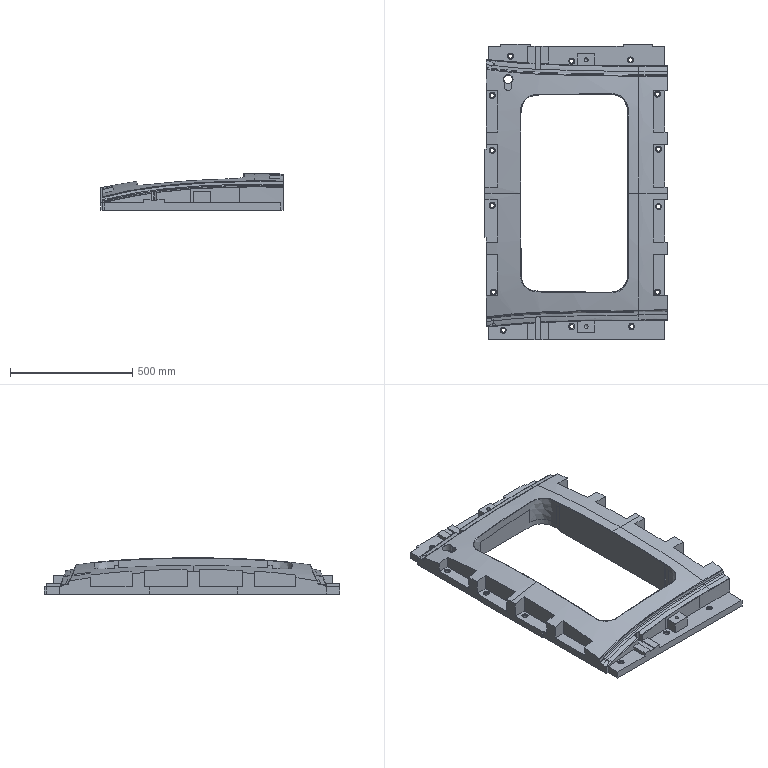Part | NX | features solid 2 | 1 solid | 234 faces | box 745 x 1210 x 148.785 mm | volume 44997379 mm3 | plane 113 | spline 82 | cylinder 37 | cone 2 | commonest cylinder face diameters 17 x14 25 x14 20 x4 16 x2 30 x1 35 x1